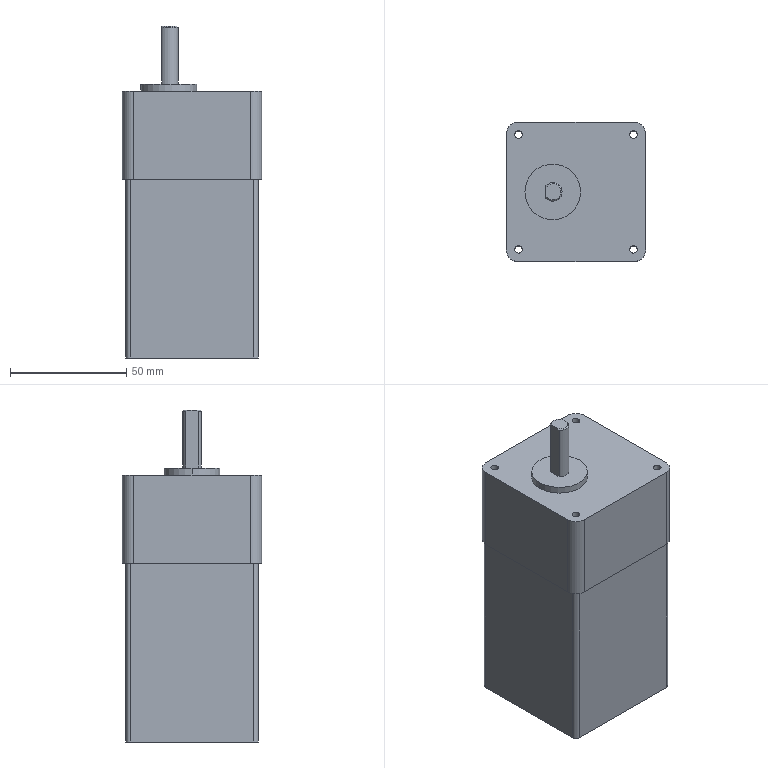Part | STEP file | 57BYG gear reduction stepper motor Mingren MR57BYG76-P10-1 | 1 solid | 34 faces | box 60 x 60 x 143 mm | volume 384480 mm3 | cylinder 19 | plane 14 | cone 1 | commonest cylinder face diameters 3.3 x8 4 x4 10 x4 24 x2 8 x1
STEP:
#1=CARTESIAN_POINT('',(-26.4,24.75,0.));
#2=VERTEX_POINT('',#1);
#3=CARTESIAN_POINT('',(-23.1,24.75,0.));
#4=VERTEX_POINT('',#3);
#5=CARTESIAN_POINT('',(-24.75,24.75,0.));
#6=DIRECTION('',(0.,0.,1.));
#7=DIRECTION('',(1.,0.,0.));
#8=AXIS2_PLACEMENT_3D('',#5,#6,#7);
#9=CIRCLE('',#8,1.65);
#10=EDGE_CURVE('',#2,#4,#9,.T.);
#11=ORIENTED_EDGE('',*,*,#10,.F.);
#12=CARTESIAN_POINT('',(-26.4,24.75,115.));
#13=VERTEX_POINT('',#12);
#14=CARTESIAN_POINT('',(-26.4,24.75,115.));
#15=DIRECTION('',(0.,0.,1.));
#16=VECTOR('',#15,1000.);
#17=LINE('',#14,#16);
#18=EDGE_CURVE('',#2,#13,#17,.T.);
#19=ORIENTED_EDGE('',*,*,#18,.T.);
#20=CARTESIAN_POINT('',(-23.1,24.75,115.));
#21=VERTEX_POINT('',#20);
#22=CARTESIAN_POINT('',(-24.75,24.75,115.));
#23=DIRECTION('',(0.,0.,1.));
#24=DIRECTION('',(1.,0.,0.));
#25=AXIS2_PLACEMENT_3D('',#22,#23,#24);
#26=CIRCLE('',#25,1.65);
#27=EDGE_CURVE('',#13,#21,#26,.T.);
#28=ORIENTED_EDGE('',*,*,#27,.T.);
#29=CARTESIAN_POINT('',(-23.1,24.75,115.));
#30=DIRECTION('',(0.,0.,1.));
#31=VECTOR('',#30,1000.);
#32=LINE('',#29,#31);
#33=EDGE_CURVE('',#4,#21,#32,.T.);
#34=ORIENTED_EDGE('',*,*,#33,.F.);
#35=EDGE_LOOP('',(#11,#19,#28,#34));
#36=FACE_OUTER_BOUND('',#35,.T.);
#37=CARTESIAN_POINT('',(-24.75,24.75,115.));
#38=DIRECTION('',(0.,0.,1.));
#39=DIRECTION('',(1.,0.,0.));
#40=AXIS2_PLACEMENT_3D('',#37,#38,#39);
#41=CYLINDRICAL_SURFACE('',#40,1.65);
#42=ADVANCED_FACE('',(#36),#41,.F.);
#43=CARTESIAN_POINT('',(23.1,24.75,0.));
#44=VERTEX_POINT('',#43);
#45=CARTESIAN_POINT('',(26.4,24.75,0.));
#46=VERTEX_POINT('',#45);
#47=CARTESIAN_POINT('',(24.75,24.75,0.));
#48=DIRECTION('',(0.,0.,1.));
#49=DIRECTION('',(1.,0.,0.));
#50=AXIS2_PLACEMENT_3D('',#47,#48,#49);
#51=CIRCLE('',#50,1.65);
#52=EDGE_CURVE('',#44,#46,#51,.T.);
#53=ORIENTED_EDGE('',*,*,#52,.F.);
#54=CARTESIAN_POINT('',(23.1,24.75,115.));
#55=VERTEX_POINT('',#54);
#56=CARTESIAN_POINT('',(23.1,24.75,115.));
#57=DIRECTION('',(0.,0.,1.));
#58=VECTOR('',#57,1000.);
#59=LINE('',#56,#58);
#60=EDGE_CURVE('',#44,#55,#59,.T.);
#61=ORIENTED_EDGE('',*,*,#60,.T.);
#62=CARTESIAN_POINT('',(26.4,24.75,115.));
#63=VERTEX_POINT('',#62);
#64=CARTESIAN_POINT('',(24.75,24.75,115.));
#65=DIRECTION('',(0.,0.,1.));
#66=DIRECTION('',(1.,0.,0.));
#67=AXIS2_PLACEMENT_3D('',#64,#65,#66);
#68=CIRCLE('',#67,1.65);
#69=EDGE_CURVE('',#55,#63,#68,.T.);
#70=ORIENTED_EDGE('',*,*,#69,.T.);
#71=CARTESIAN_POINT('',(26.4,24.75,115.));
#72=DIRECTION('',(0.,0.,1.));
#73=VECTOR('',#72,1000.);
#74=LINE('',#71,#73);
#75=EDGE_CURVE('',#46,#63,#74,.T.);
#76=ORIENTED_EDGE('',*,*,#75,.F.);
#77=EDGE_LOOP('',(#53,#61,#70,#76));
#78=FACE_OUTER_BOUND('',#77,.T.);
#79=CARTESIAN_POINT('',(24.75,24.75,115.));
#80=DIRECTION('',(0.,0.,1.));
#81=DIRECTION('',(1.,0.,0.));
#82=AXIS2_PLACEMENT_3D('',#79,#80,#81);
#83=CYLINDRICAL_SURFACE('',#82,1.65);
#84=ADVANCED_FACE('',(#78),#83,.F.);
#85=CARTESIAN_POINT('',(23.1,-24.75,0.));
#86=VERTEX_POINT('',#85);
#87=CARTESIAN_POINT('',(26.4,-24.75,0.));
#88=VERTEX_POINT('',#87);
#89=CARTESIAN_POINT('',(24.75,-24.75,0.));
#90=DIRECTION('',(0.,0.,1.));
#91=DIRECTION('',(1.,0.,0.));
#92=AXIS2_PLACEMENT_3D('',#89,#90,#91);
#93=CIRCLE('',#92,1.65);
#94=EDGE_CURVE('',#86,#88,#93,.T.);
#95=ORIENTED_EDGE('',*,*,#94,.F.);
#96=CARTESIAN_POINT('',(23.1,-24.75,115.));
#97=VERTEX_POINT('',#96);
#98=CARTESIAN_POINT('',(23.1,-24.75,115.));
#99=DIRECTION('',(0.,0.,1.));
#100=VECTOR('',#99,1000.);
#101=LINE('',#98,#100);
#102=EDGE_CURVE('',#86,#97,#101,.T.);
#103=ORIENTED_EDGE('',*,*,#102,.T.);
#104=CARTESIAN_POINT('',(26.4,-24.75,115.));
#105=VERTEX_POINT('',#104);
#106=CARTESIAN_POINT('',(24.75,-24.75,115.));
#107=DIRECTION('',(0.,0.,1.));
#108=DIRECTION('',(1.,0.,0.));
#109=AXIS2_PLACEMENT_3D('',#106,#107,#108);
#110=CIRCLE('',#109,1.65);
#111=EDGE_CURVE('',#97,#105,#110,.T.);
#112=ORIENTED_EDGE('',*,*,#111,.T.);
#113=CARTESIAN_POINT('',(26.4,-24.75,115.));
#114=DIRECTION('',(0.,0.,1.));
#115=VECTOR('',#114,1000.);
#116=LINE('',#113,#115);
#117=EDGE_CURVE('',#88,#105,#116,.T.);
#118=ORIENTED_EDGE('',*,*,#117,.F.);
#119=EDGE_LOOP('',(#95,#103,#112,#118));
#120=FACE_OUTER_BOUND('',#119,.T.);
#121=CARTESIAN_POINT('',(24.75,-24.75,115.));
#122=DIRECTION('',(0.,0.,1.));
#123=DIRECTION('',(1.,0.,0.));
#124=AXIS2_PLACEMENT_3D('',#121,#122,#123);
#125=CYLINDRICAL_SURFACE('',#124,1.65);
#126=ADVANCED_FACE('',(#120),#125,.F.);
#127=CARTESIAN_POINT('',(-26.4,-24.75,0.));
#128=VERTEX_POINT('',#127);
#129=CARTESIAN_POINT('',(-23.1,-24.75,0.));
#130=VERTEX_POINT('',#129);
#131=CARTESIAN_POINT('',(-24.75,-24.75,0.));
#132=DIRECTION('',(0.,0.,1.));
#133=DIRECTION('',(1.,0.,0.));
#134=AXIS2_PLACEMENT_3D('',#131,#132,#133);
#135=CIRCLE('',#134,1.65);
#136=EDGE_CURVE('',#128,#130,#135,.T.);
#137=ORIENTED_EDGE('',*,*,#136,.F.);
#138=CARTESIAN_POINT('',(-26.4,-24.75,115.));
#139=VERTEX_POINT('',#138);
#140=CARTESIAN_POINT('',(-26.4,-24.75,115.));
#141=DIRECTION('',(0.,0.,1.));
#142=VECTOR('',#141,1000.);
#143=LINE('',#140,#142);
#144=EDGE_CURVE('',#128,#139,#143,.T.);
#145=ORIENTED_EDGE('',*,*,#144,.T.);
#146=CARTESIAN_POINT('',(-23.1,-24.75,115.));
#147=VERTEX_POINT('',#146);
#148=CARTESIAN_POINT('',(-24.75,-24.75,115.));
#149=DIRECTION('',(0.,0.,1.));
#150=DIRECTION('',(1.,0.,0.));
#151=AXIS2_PLACEMENT_3D('',#148,#149,#150);
#152=CIRCLE('',#151,1.65);
#153=EDGE_CURVE('',#139,#147,#152,.T.);
#154=ORIENTED_EDGE('',*,*,#153,.T.);
#155=CARTESIAN_POINT('',(-23.1,-24.75,115.));
#156=DIRECTION('',(0.,0.,1.));
#157=VECTOR('',#156,1000.);
#158=LINE('',#155,#157);
#159=EDGE_CURVE('',#130,#147,#158,.T.);
#160=ORIENTED_EDGE('',*,*,#159,.F.);
#161=EDGE_LOOP('',(#137,#145,#154,#160));
#162=FACE_OUTER_BOUND('',#161,.T.);
#163=CARTESIAN_POINT('',(-24.75,-24.75,115.));
#164=DIRECTION('',(0.,0.,1.));
#165=DIRECTION('',(1.,0.,0.));
#166=AXIS2_PLACEMENT_3D('',#163,#164,#165);
#167=CYLINDRICAL_SURFACE('',#166,1.65);
#168=ADVANCED_FACE('',(#162),#167,.F.);
#169=CARTESIAN_POINT('',(2.,0.,118.));
#170=VERTEX_POINT('',#169);
#171=CARTESIAN_POINT('',(-22.,0.,118.));
#172=VERTEX_POINT('',#171);
#173=CARTESIAN_POINT('',(-10.,0.,118.));
#174=DIRECTION('',(0.,0.,1.));
#175=DIRECTION('',(1.,0.,0.));
#176=AXIS2_PLACEMENT_3D('',#173,#174,#175);
#177=CIRCLE('',#176,12.);
#178=EDGE_CURVE('',#170,#172,#177,.T.);
#179=ORIENTED_EDGE('',*,*,#178,.F.);
#180=CARTESIAN_POINT('',(2.,0.,115.));
#181=VERTEX_POINT('',#180);
#182=CARTESIAN_POINT('',(2.,0.,118.));
#183=DIRECTION('',(0.,0.,-1.));
#184=VECTOR('',#183,1000.);
#185=LINE('',#182,#184);
#186=EDGE_CURVE('',#170,#181,#185,.T.);
#187=ORIENTED_EDGE('',*,*,#186,.T.);
#188=CARTESIAN_POINT('',(-22.,0.,115.));
#189=VERTEX_POINT('',#188);
#190=CARTESIAN_POINT('',(-10.,0.,115.));
#191=DIRECTION('',(0.,0.,1.));
#192=DIRECTION('',(1.,0.,0.));
#193=AXIS2_PLACEMENT_3D('',#190,#191,#192);
#194=CIRCLE('',#193,12.);
#195=EDGE_CURVE('',#181,#189,#194,.T.);
#196=ORIENTED_EDGE('',*,*,#195,.T.);
#197=CARTESIAN_POINT('',(-22.,0.,118.));
#198=DIRECTION('',(0.,0.,-1.));
#199=VECTOR('',#198,1000.);
#200=LINE('',#197,#199);
#201=EDGE_CURVE('',#172,#189,#200,.T.);
#202=ORIENTED_EDGE('',*,*,#201,.F.);
#203=EDGE_LOOP('',(#179,#187,#196,#202));
#204=FACE_OUTER_BOUND('',#203,.T.);
#205=CARTESIAN_POINT('',(-10.,0.,118.));
#206=DIRECTION('',(0.,0.,-1.));
#207=DIRECTION('',(-1.,0.,0.));
#208=AXIS2_PLACEMENT_3D('',#205,#206,#207);
#209=CYLINDRICAL_SURFACE('',#208,12.);
#210=ADVANCED_FACE('',(#204),#209,.T.);
#211=CARTESIAN_POINT('',(-30.,-25.,77.));
#212=VERTEX_POINT('',#211);
#213=CARTESIAN_POINT('',(-30.,25.,77.));
#214=VERTEX_POINT('',#213);
#215=CARTESIAN_POINT('',(-30.,30.,77.));
#216=DIRECTION('',(0.,1.,0.));
#217=VECTOR('',#216,1000.);
#218=LINE('',#215,#217);
#219=EDGE_CURVE('',#212,#214,#218,.T.);
#220=ORIENTED_EDGE('',*,*,#219,.F.);
#221=CARTESIAN_POINT('',(-30.,-25.,115.));
#222=VERTEX_POINT('',#221);
#223=CARTESIAN_POINT('',(-30.,-25.,115.));
#224=DIRECTION('',(0.,0.,1.));
#225=VECTOR('',#224,1000.);
#226=LINE('',#223,#225);
#227=EDGE_CURVE('',#212,#222,#226,.T.);
#228=ORIENTED_EDGE('',*,*,#227,.T.);
#229=CARTESIAN_POINT('',(-30.,25.,115.));
#230=VERTEX_POINT('',#229);
#231=CARTESIAN_POINT('',(-30.,30.,115.));
#232=DIRECTION('',(0.,-1.,0.));
#233=VECTOR('',#232,1000.);
#234=LINE('',#231,#233);
#235=EDGE_CURVE('',#230,#222,#234,.T.);
#236=ORIENTED_EDGE('',*,*,#235,.F.);
#237=CARTESIAN_POINT('',(-30.,25.,115.));
#238=DIRECTION('',(0.,0.,-1.));
#239=VECTOR('',#238,1000.);
#240=LINE('',#237,#239);
#241=EDGE_CURVE('',#230,#214,#240,.T.);
#242=ORIENTED_EDGE('',*,*,#241,.T.);
#243=EDGE_LOOP('',(#220,#228,#236,#242));
#244=FACE_OUTER_BOUND('',#243,.T.);
#245=CARTESIAN_POINT('',(-30.,30.,115.));
#246=DIRECTION('',(1.,0.,0.));
#247=DIRECTION('',(0.,0.,-1.));
#248=AXIS2_PLACEMENT_3D('',#245,#246,#247);
#249=PLANE('',#248);
#250=ADVANCED_FACE('',(#244),#249,.F.);
#251=CARTESIAN_POINT('',(25.,-30.,77.));
#252=VERTEX_POINT('',#251);
#253=CARTESIAN_POINT('',(-25.,-30.,77.));
#254=VERTEX_POINT('',#253);
#255=CARTESIAN_POINT('',(-30.,-30.,77.));
#256=DIRECTION('',(-1.,0.,0.));
#257=VECTOR('',#256,1000.);
#258=LINE('',#255,#257);
#259=EDGE_CURVE('',#252,#254,#258,.T.);
#260=ORIENTED_EDGE('',*,*,#259,.F.);
#261=CARTESIAN_POINT('',(25.,-30.,115.));
#262=VERTEX_POINT('',#261);
#263=CARTESIAN_POINT('',(25.,-30.,115.));
#264=DIRECTION('',(0.,0.,1.));
#265=VECTOR('',#264,1000.);
#266=LINE('',#263,#265);
#267=EDGE_CURVE('',#252,#262,#266,.T.);
#268=ORIENTED_EDGE('',*,*,#267,.T.);
#269=CARTESIAN_POINT('',(-25.,-30.,115.));
#270=VERTEX_POINT('',#269);
#271=CARTESIAN_POINT('',(-30.,-30.,115.));
#272=DIRECTION('',(1.,0.,0.));
#273=VECTOR('',#272,1000.);
#274=LINE('',#271,#273);
#275=EDGE_CURVE('',#270,#262,#274,.T.);
#276=ORIENTED_EDGE('',*,*,#275,.F.);
#277=CARTESIAN_POINT('',(-25.,-30.,115.));
#278=DIRECTION('',(0.,0.,-1.));
#279=VECTOR('',#278,1000.);
#280=LINE('',#277,#279);
#281=EDGE_CURVE('',#270,#254,#280,.T.);
#282=ORIENTED_EDGE('',*,*,#281,.T.);
#283=EDGE_LOOP('',(#260,#268,#276,#282));
#284=FACE_OUTER_BOUND('',#283,.T.);
#285=CARTESIAN_POINT('',(-30.,-30.,115.));
#286=DIRECTION('',(0.,1.,0.));
#287=DIRECTION('',(0.,0.,1.));
#288=AXIS2_PLACEMENT_3D('',#285,#286,#287);
#289=PLANE('',#288);
#290=ADVANCED_FACE('',(#284),#289,.F.);
#291=CARTESIAN_POINT('',(30.,25.,77.));
#292=VERTEX_POINT('',#291);
#293=CARTESIAN_POINT('',(30.,-25.,77.));
#294=VERTEX_POINT('',#293);
#295=CARTESIAN_POINT('',(30.,30.,77.));
#296=DIRECTION('',(0.,-1.,0.));
#297=VECTOR('',#296,1000.);
#298=LINE('',#295,#297);
#299=EDGE_CURVE('',#292,#294,#298,.T.);
#300=ORIENTED_EDGE('',*,*,#299,.F.);
#301=CARTESIAN_POINT('',(30.,25.,115.));
#302=VERTEX_POINT('',#301);
#303=CARTESIAN_POINT('',(30.,25.,115.));
#304=DIRECTION('',(0.,0.,1.));
#305=VECTOR('',#304,1000.);
#306=LINE('',#303,#305);
#307=EDGE_CURVE('',#292,#302,#306,.T.);
#308=ORIENTED_EDGE('',*,*,#307,.T.);
#309=CARTESIAN_POINT('',(30.,-25.,115.));
#310=VERTEX_POINT('',#309);
#311=CARTESIAN_POINT('',(30.,30.,115.));
#312=DIRECTION('',(0.,1.,0.));
#313=VECTOR('',#312,1000.);
#314=LINE('',#311,#313);
#315=EDGE_CURVE('',#310,#302,#314,.T.);
#316=ORIENTED_EDGE('',*,*,#315,.F.);
#317=CARTESIAN_POINT('',(30.,-25.,115.));
#318=DIRECTION('',(0.,0.,-1.));
#319=VECTOR('',#318,1000.);
#320=LINE('',#317,#319);
#321=EDGE_CURVE('',#310,#294,#320,.T.);
#322=ORIENTED_EDGE('',*,*,#321,.T.);
#323=EDGE_LOOP('',(#300,#308,#316,#322));
#324=FACE_OUTER_BOUND('',#323,.T.);
#325=CARTESIAN_POINT('',(30.,30.,115.));
#326=DIRECTION('',(-1.,0.,0.));
#327=DIRECTION('',(0.,0.,1.));
#328=AXIS2_PLACEMENT_3D('',#325,#326,#327);
#329=PLANE('',#328);
#330=ADVANCED_FACE('',(#324),#329,.F.);
#331=CARTESIAN_POINT('',(-25.,30.,77.));
#332=VERTEX_POINT('',#331);
#333=CARTESIAN_POINT('',(25.,30.,77.));
#334=VERTEX_POINT('',#333);
#335=CARTESIAN_POINT('',(-30.,30.,77.));
#336=DIRECTION('',(1.,0.,0.));
#337=VECTOR('',#336,1000.);
#338=LINE('',#335,#337);
#339=EDGE_CURVE('',#332,#334,#338,.T.);
#340=ORIENTED_EDGE('',*,*,#339,.F.);
#341=CARTESIAN_POINT('',(-25.,30.,115.));
#342=VERTEX_POINT('',#341);
#343=CARTESIAN_POINT('',(-25.,30.,115.));
#344=DIRECTION('',(0.,0.,1.));
#345=VECTOR('',#344,1000.);
#346=LINE('',#343,#345);
#347=EDGE_CURVE('',#332,#342,#346,.T.);
#348=ORIENTED_EDGE('',*,*,#347,.T.);
#349=CARTESIAN_POINT('',(25.,30.,115.));
#350=VERTEX_POINT('',#349);
#351=CARTESIAN_POINT('',(-30.,30.,115.));
#352=DIRECTION('',(-1.,0.,0.));
#353=VECTOR('',#352,1000.);
#354=LINE('',#351,#353);
#355=EDGE_CURVE('',#350,#342,#354,.T.);
#356=ORIENTED_EDGE('',*,*,#355,.F.);
#357=CARTESIAN_POINT('',(25.,30.,115.));
#358=DIRECTION('',(0.,0.,-1.));
#359=VECTOR('',#358,1000.);
#360=LINE('',#357,#359);
#361=EDGE_CURVE('',#350,#334,#360,.T.);
#362=ORIENTED_EDGE('',*,*,#361,.T.);
#363=EDGE_LOOP('',(#340,#348,#356,#362));
#364=FACE_OUTER_BOUND('',#363,.T.);
#365=CARTESIAN_POINT('',(-30.,30.,115.));
#366=DIRECTION('',(0.,-1.,0.));
#367=DIRECTION('',(0.,0.,-1.));
#368=AXIS2_PLACEMENT_3D('',#365,#366,#367);
#369=PLANE('',#368);
#370=ADVANCED_FACE('',(#364),#369,.F.);
#371=ORIENTED_EDGE('',*,*,#227,.F.);
#372=CARTESIAN_POINT('',(-25.,-25.,77.));
#373=DIRECTION('',(0.,0.,1.));
#374=DIRECTION('',(-1.,0.,0.));
#375=AXIS2_PLACEMENT_3D('',#372,#373,#374);
#376=CIRCLE('',#375,5.);
#377=EDGE_CURVE('',#212,#254,#376,.T.);
#378=ORIENTED_EDGE('',*,*,#377,.T.);
#379=ORIENTED_EDGE('',*,*,#281,.F.);
#380=CARTESIAN_POINT('',(-25.,-25.,115.));
#381=DIRECTION('',(0.,0.,1.));
#382=DIRECTION('',(1.,0.,0.));
#383=AXIS2_PLACEMENT_3D('',#380,#381,#382);
#384=CIRCLE('',#383,5.);
#385=EDGE_CURVE('',#222,#270,#384,.T.);
#386=ORIENTED_EDGE('',*,*,#385,.F.);
#387=EDGE_LOOP('',(#371,#378,#379,#386));
#388=FACE_OUTER_BOUND('',#387,.T.);
#389=CARTESIAN_POINT('',(-25.,-25.,115.));
#390=DIRECTION('',(0.,0.,-1.));
#391=DIRECTION('',(-1.,0.,0.));
#392=AXIS2_PLACEMENT_3D('',#389,#390,#391);
#393=CYLINDRICAL_SURFACE('',#392,5.);
#394=ADVANCED_FACE('',(#388),#393,.T.);
#395=ORIENTED_EDGE('',*,*,#267,.F.);
#396=CARTESIAN_POINT('',(25.,-25.,77.));
#397=DIRECTION('',(0.,0.,1.));
#398=DIRECTION('',(-1.,0.,0.));
#399=AXIS2_PLACEMENT_3D('',#396,#397,#398);
#400=CIRCLE('',#399,5.);
#401=EDGE_CURVE('',#252,#294,#400,.T.);
#402=ORIENTED_EDGE('',*,*,#401,.T.);
#403=ORIENTED_EDGE('',*,*,#321,.F.);
#404=CARTESIAN_POINT('',(25.,-25.,115.));
#405=DIRECTION('',(0.,0.,1.));
#406=DIRECTION('',(1.,0.,0.));
#407=AXIS2_PLACEMENT_3D('',#404,#405,#406);
#408=CIRCLE('',#407,5.);
#409=EDGE_CURVE('',#262,#310,#408,.T.);
#410=ORIENTED_EDGE('',*,*,#409,.F.);
#411=EDGE_LOOP('',(#395,#402,#403,#410));
#412=FACE_OUTER_BOUND('',#411,.T.);
#413=CARTESIAN_POINT('',(25.,-25.,115.));
#414=DIRECTION('',(0.,0.,-1.));
#415=DIRECTION('',(-1.,0.,0.));
#416=AXIS2_PLACEMENT_3D('',#413,#414,#415);
#417=CYLINDRICAL_SURFACE('',#416,5.);
#418=ADVANCED_FACE('',(#412),#417,.T.);
#419=ORIENTED_EDGE('',*,*,#307,.F.);
#420=CARTESIAN_POINT('',(25.,25.,77.));
#421=DIRECTION('',(0.,0.,1.));
#422=DIRECTION('',(-1.,0.,0.));
#423=AXIS2_PLACEMENT_3D('',#420,#421,#422);
#424=CIRCLE('',#423,5.);
#425=EDGE_CURVE('',#292,#334,#424,.T.);
#426=ORIENTED_EDGE('',*,*,#425,.T.);
#427=ORIENTED_EDGE('',*,*,#361,.F.);
#428=CARTESIAN_POINT('',(25.,25.,115.));
#429=DIRECTION('',(0.,0.,1.));
#430=DIRECTION('',(1.,0.,0.));
#431=AXIS2_PLACEMENT_3D('',#428,#429,#430);
#432=CIRCLE('',#431,5.);
#433=EDGE_CURVE('',#302,#350,#432,.T.);
#434=ORIENTED_EDGE('',*,*,#433,.F.);
#435=EDGE_LOOP('',(#419,#426,#427,#434));
#436=FACE_OUTER_BOUND('',#435,.T.);
#437=CARTESIAN_POINT('',(25.,25.,115.));
#438=DIRECTION('',(0.,0.,-1.));
#439=DIRECTION('',(-1.,0.,0.));
#440=AXIS2_PLACEMENT_3D('',#437,#438,#439);
#441=CYLINDRICAL_SURFACE('',#440,5.);
#442=ADVANCED_FACE('',(#436),#441,.T.);
#443=ORIENTED_EDGE('',*,*,#347,.F.);
#444=CARTESIAN_POINT('',(-25.,25.,77.));
#445=DIRECTION('',(0.,0.,1.));
#446=DIRECTION('',(-1.,0.,0.));
#447=AXIS2_PLACEMENT_3D('',#444,#445,#446);
#448=CIRCLE('',#447,5.);
#449=EDGE_CURVE('',#332,#214,#448,.T.);
#450=ORIENTED_EDGE('',*,*,#449,.T.);
#451=ORIENTED_EDGE('',*,*,#241,.F.);
#452=CARTESIAN_POINT('',(-25.,25.,115.));
#453=DIRECTION('',(0.,0.,1.));
#454=DIRECTION('',(1.,0.,0.));
#455=AXIS2_PLACEMENT_3D('',#452,#453,#454);
#456=CIRCLE('',#455,5.);
#457=EDGE_CURVE('',#342,#230,#456,.T.);
#458=ORIENTED_EDGE('',*,*,#457,.F.);
#459=EDGE_LOOP('',(#443,#450,#451,#458));
#460=FACE_OUTER_BOUND('',#459,.T.);
#461=CARTESIAN_POINT('',(-25.,25.,115.));
#462=DIRECTION('',(0.,0.,-1.));
#463=DIRECTION('',(-1.,0.,0.));
#464=AXIS2_PLACEMENT_3D('',#461,#462,#463);
#465=CYLINDRICAL_SURFACE('',#464,5.);
#466=ADVANCED_FACE('',(#460),#465,.T.);
#467=CARTESIAN_POINT('',(-24.75,24.75,115.));
#468=DIRECTION('',(0.,0.,1.));
#469=DIRECTION('',(1.,0.,0.));
#470=AXIS2_PLACEMENT_3D('',#467,#468,#469);
#471=CIRCLE('',#470,1.65);
#472=EDGE_CURVE('',#21,#13,#471,.T.);
#473=ORIENTED_EDGE('',*,*,#472,.F.);
#474=ORIENTED_EDGE('',*,*,#27,.F.);
#475=EDGE_LOOP('',(#473,#474));
#476=FACE_BOUND('',#475,.T.);
#477=CARTESIAN_POINT('',(24.75,24.75,115.));
#478=DIRECTION('',(0.,0.,1.));
#479=DIRECTION('',(1.,0.,0.));
#480=AXIS2_PLACEMENT_3D('',#477,#478,#479);
#481=CIRCLE('',#480,1.65);
#482=EDGE_CURVE('',#63,#55,#481,.T.);
#483=ORIENTED_EDGE('',*,*,#482,.F.);
#484=ORIENTED_EDGE('',*,*,#69,.F.);
#485=EDGE_LOOP('',(#483,#484));
#486=FACE_BOUND('',#485,.T.);
#487=CARTESIAN_POINT('',(24.75,-24.75,115.));
#488=DIRECTION('',(0.,0.,1.));
#489=DIRECTION('',(1.,0.,0.));
#490=AXIS2_PLACEMENT_3D('',#487,#488,#489);
#491=CIRCLE('',#490,1.65);
#492=EDGE_CURVE('',#105,#97,#491,.T.);
#493=ORIENTED_EDGE('',*,*,#492,.F.);
#494=ORIENTED_EDGE('',*,*,#111,.F.);
#495=EDGE_LOOP('',(#493,#494));
#496=FACE_BOUND('',#495,.T.);
#497=CARTESIAN_POINT('',(-24.75,-24.75,115.));
#498=DIRECTION('',(0.,0.,1.));
#499=DIRECTION('',(1.,0.,0.));
#500=AXIS2_PLACEMENT_3D('',#497,#498,#499);
#501=CIRCLE('',#500,1.65);
#502=EDGE_CURVE('',#147,#139,#501,.T.);
#503=ORIENTED_EDGE('',*,*,#502,.F.);
#504=ORIENTED_EDGE('',*,*,#153,.F.);
#505=EDGE_LOOP('',(#503,#504));
#506=FACE_BOUND('',#505,.T.);
#507=ORIENTED_EDGE('',*,*,#235,.T.);
#508=ORIENTED_EDGE('',*,*,#385,.T.);
#509=ORIENTED_EDGE('',*,*,#275,.T.);
#510=ORIENTED_EDGE('',*,*,#409,.T.);
#511=ORIENTED_EDGE('',*,*,#315,.T.);
#512=ORIENTED_EDGE('',*,*,#433,.T.);
#513=ORIENTED_EDGE('',*,*,#355,.T.);
#514=ORIENTED_EDGE('',*,*,#457,.T.);
#515=EDGE_LOOP('',(#507,#508,#509,#510,#511,#512,#513,#514));
#516=FACE_OUTER_BOUND('',#515,.T.);
#517=CARTESIAN_POINT('',(-10.,0.,115.));
#518=DIRECTION('',(0.,0.,1.));
#519=DIRECTION('',(1.,0.,0.));
#520=AXIS2_PLACEMENT_3D('',#517,#518,#519);
#521=CIRCLE('',#520,12.);
#522=EDGE_CURVE('',#189,#181,#521,.T.);
#523=ORIENTED_EDGE('',*,*,#522,.F.);
#524=ORIENTED_EDGE('',*,*,#195,.F.);
#525=EDGE_LOOP('',(#523,#524));
#526=FACE_BOUND('',#525,.T.);
#527=CARTESIAN_POINT('',(-30.,-30.,115.));
#528=DIRECTION('',(0.,0.,1.));
#529=DIRECTION('',(1.,0.,0.));
#530=AXIS2_PLACEMENT_3D('',#527,#528,#529);
#531=PLANE('',#530);
#532=ADVANCED_FACE('',(#476,#486,#496,#506,#516,#526),#531,.T.);
#533=CARTESIAN_POINT('',(-13.,-2.646,118.));
#534=VERTEX_POINT('',#533);
#535=CARTESIAN_POINT('',(-13.,2.646,118.));
#536=VERTEX_POINT('',#535);
#537=CARTESIAN_POINT('',(-10.,0.,118.));
#538=DIRECTION('',(0.,0.,1.));
#539=DIRECTION('',(1.,0.,0.));
#540=AXIS2_PLACEMENT_3D('',#537,#538,#539);
#541=CIRCLE('',#540,4.);
#542=EDGE_CURVE('',#534,#536,#541,.T.);
#543=ORIENTED_EDGE('',*,*,#542,.F.);
#544=CARTESIAN_POINT('',(-13.,5.,118.));
#545=DIRECTION('',(0.,1.,0.));
#546=VECTOR('',#545,1000.);
#547=LINE('',#544,#546);
#548=EDGE_CURVE('',#534,#536,#547,.T.);
#549=ORIENTED_EDGE('',*,*,#548,.T.);
#550=EDGE_LOOP('',(#543,#549));
#551=FACE_BOUND('',#550,.T.);
#552=CARTESIAN_POINT('',(-10.,0.,118.));
#553=DIRECTION('',(0.,0.,1.));
#554=DIRECTION('',(1.,0.,0.));
#555=AXIS2_PLACEMENT_3D('',#552,#553,#554);
#556=CIRCLE('',#555,12.);
#557=EDGE_CURVE('',#172,#170,#556,.T.);
#558=ORIENTED_EDGE('',*,*,#557,.T.);
#559=ORIENTED_EDGE('',*,*,#178,.T.);
#560=EDGE_LOOP('',(#558,#559));
#561=FACE_OUTER_BOUND('',#560,.T.);
#562=CARTESIAN_POINT('',(-10.,0.,118.));
#563=DIRECTION('',(0.,0.,1.));
#564=DIRECTION('',(1.,0.,0.));
#565=AXIS2_PLACEMENT_3D('',#562,#563,#564);
#566=PLANE('',#565);
#567=ADVANCED_FACE('',(#551,#561),#566,.T.);
#568=ORIENTED_EDGE('',*,*,#186,.F.);
#569=ORIENTED_EDGE('',*,*,#557,.F.);
#570=ORIENTED_EDGE('',*,*,#201,.T.);
#571=ORIENTED_EDGE('',*,*,#522,.T.);
#572=EDGE_LOOP('',(#568,#569,#570,#571));
#573=FACE_OUTER_BOUND('',#572,.T.);
#574=CARTESIAN_POINT('',(-10.,0.,118.));
#575=DIRECTION('',(0.,0.,-1.));
#576=DIRECTION('',(-1.,0.,0.));
#577=AXIS2_PLACEMENT_3D('',#574,#575,#576);
#578=CYLINDRICAL_SURFACE('',#577,12.);
#579=ADVANCED_FACE('',(#573),#578,.T.);
#580=CARTESIAN_POINT('',(-13.,-1.803,143.));
#581=VERTEX_POINT('',#580);
#582=CARTESIAN_POINT('',(-13.,1.803,143.));
#583=VERTEX_POINT('',#582);
#584=CARTESIAN_POINT('',(-13.,5.,143.));
#585=DIRECTION('',(0.,1.,0.));
#586=VECTOR('',#585,1000.);
#587=LINE('',#584,#586);
#588=EDGE_CURVE('',#581,#583,#587,.T.);
#589=ORIENTED_EDGE('',*,*,#588,.F.);
#590=CARTESIAN_POINT('',(-10.,0.,143.));
#591=DIRECTION('',(0.,0.,1.));
#592=DIRECTION('',(1.,0.,0.));
#593=AXIS2_PLACEMENT_3D('',#590,#591,#592);
#594=CIRCLE('',#593,3.5);
#595=EDGE_CURVE('',#581,#583,#594,.T.);
#596=ORIENTED_EDGE('',*,*,#595,.T.);
#597=EDGE_LOOP('',(#589,#596));
#598=FACE_OUTER_BOUND('',#597,.T.);
#599=CARTESIAN_POINT('',(-10.,0.,143.));
#600=DIRECTION('',(0.,0.,1.));
#601=DIRECTION('',(1.,0.,0.));
#602=AXIS2_PLACEMENT_3D('',#599,#600,#601);
#603=PLANE('',#602);
#604=ADVANCED_FACE('',(#598),#603,.T.);
#605=CARTESIAN_POINT('',(-13.,2.646,142.5));
#606=VERTEX_POINT('',#605);
#607=CARTESIAN_POINT('',(-13.,-2.646,142.5));
#608=VERTEX_POINT('',#607);
#609=CARTESIAN_POINT('',(-10.,0.,142.5));
#610=DIRECTION('',(0.,0.,-1.));
#611=DIRECTION('',(1.,0.,0.));
#612=AXIS2_PLACEMENT_3D('',#609,#610,#611);
#613=CIRCLE('',#612,4.);
#614=EDGE_CURVE('',#606,#608,#613,.T.);
#615=ORIENTED_EDGE('',*,*,#614,.T.);
#616=CARTESIAN_POINT('',(-13.,-2.646,143.));
#617=DIRECTION('',(0.,0.,-1.));
#618=VECTOR('',#617,1000.);
#619=LINE('',#616,#618);
#620=EDGE_CURVE('',#608,#534,#619,.T.);
#621=ORIENTED_EDGE('',*,*,#620,.T.);
#622=ORIENTED_EDGE('',*,*,#542,.T.);
#623=CARTESIAN_POINT('',(-13.,2.646,143.));
#624=DIRECTION('',(0.,0.,1.));
#625=VECTOR('',#624,1000.);
#626=LINE('',#623,#625);
#627=EDGE_CURVE('',#536,#606,#626,.T.);
#628=ORIENTED_EDGE('',*,*,#627,.T.);
#629=EDGE_LOOP('',(#615,#621,#622,#628));
#630=FACE_OUTER_BOUND('',#629,.T.);
#631=CARTESIAN_POINT('',(-10.,0.,143.));
#632=DIRECTION('',(0.,0.,-1.));
#633=DIRECTION('',(-1.,0.,0.));
#634=AXIS2_PLACEMENT_3D('',#631,#632,#633);
#635=CYLINDRICAL_SURFACE('',#634,4.);
#636=ADVANCED_FACE('',(#630),#635,.T.);
#637=CARTESIAN_POINT('',(-13.,-2.646,142.5));
#638=CARTESIAN_POINT('',(-13.,-2.374,142.68));
#639=CARTESIAN_POINT('',(-13.,-2.095,142.849));
#640=CARTESIAN_POINT('',(-13.,-1.803,143.));
#641=B_SPLINE_CURVE_WITH_KNOTS('',3,(#637,#638,#639,#640),.UNSPECIFIED.,.F.,.F.,(4,4),(0.007424,0.008405),.UNSPECIFIED.);
#642=EDGE_CURVE('',#608,#581,#641,.T.);
#643=ORIENTED_EDGE('',*,*,#642,.F.);
#644=ORIENTED_EDGE('',*,*,#614,.F.);
#645=CARTESIAN_POINT('',(-13.,1.803,143.));
#646=CARTESIAN_POINT('',(-13.,2.092,142.851));
#647=CARTESIAN_POINT('',(-13.,2.373,142.68));
#648=CARTESIAN_POINT('',(-13.,2.646,142.5));
#649=B_SPLINE_CURVE_WITH_KNOTS('',3,(#645,#646,#647,#648),.UNSPECIFIED.,.F.,.F.,(4,4),(0.01215,0.01313),.UNSPECIFIED.);
#650=EDGE_CURVE('',#583,#606,#649,.T.);
#651=ORIENTED_EDGE('',*,*,#650,.F.);
#652=ORIENTED_EDGE('',*,*,#595,.F.);
#653=EDGE_LOOP('',(#643,#644,#651,#652));
#654=FACE_OUTER_BOUND('',#653,.T.);
#655=CARTESIAN_POINT('',(-10.,0.,143.));
#656=DIRECTION('',(0.,0.,-1.));
#657=DIRECTION('',(-1.,0.,0.));
#658=AXIS2_PLACEMENT_3D('',#655,#656,#657);
#659=CONICAL_SURFACE('',#658,3.5,0.7854);
#660=ADVANCED_FACE('',(#654),#659,.T.);
#661=ORIENTED_EDGE('',*,*,#642,.T.);
#662=ORIENTED_EDGE('',*,*,#588,.T.);
#663=ORIENTED_EDGE('',*,*,#650,.T.);
#664=ORIENTED_EDGE('',*,*,#627,.F.);
#665=ORIENTED_EDGE('',*,*,#548,.F.);
#666=ORIENTED_EDGE('',*,*,#620,.F.);
#667=EDGE_LOOP('',(#661,#662,#663,#664,#665,#666));
#668=FACE_OUTER_BOUND('',#667,.T.);
#669=CARTESIAN_POINT('',(-13.,5.,118.));
#670=DIRECTION('',(1.,0.,0.));
#671=DIRECTION('',(0.,0.,-1.));
#672=AXIS2_PLACEMENT_3D('',#669,#670,#671);
#673=PLANE('',#672);
#674=ADVANCED_FACE('',(#668),#673,.F.);
#675=ORIENTED_EDGE('',*,*,#259,.T.);
#676=ORIENTED_EDGE('',*,*,#377,.F.);
#677=ORIENTED_EDGE('',*,*,#219,.T.);
#678=ORIENTED_EDGE('',*,*,#449,.F.);
#679=ORIENTED_EDGE('',*,*,#339,.T.);
#680=ORIENTED_EDGE('',*,*,#425,.F.);
#681=ORIENTED_EDGE('',*,*,#299,.T.);
#682=ORIENTED_EDGE('',*,*,#401,.F.);
#683=EDGE_LOOP('',(#675,#676,#677,#678,#679,#680,#681,#682));
#684=FACE_OUTER_BOUND('',#683,.T.);
#685=CARTESIAN_POINT('',(26.5,-28.5,77.));
#686=VERTEX_POINT('',#685);
#687=CARTESIAN_POINT('',(-26.5,-28.5,77.));
#688=VERTEX_POINT('',#687);
#689=CARTESIAN_POINT('',(28.5,-28.5,77.));
#690=DIRECTION('',(-1.,0.,0.));
#691=VECTOR('',#690,1000.);
#692=LINE('',#689,#691);
#693=EDGE_CURVE('',#686,#688,#692,.T.);
#694=ORIENTED_EDGE('',*,*,#693,.F.);
#695=CARTESIAN_POINT('',(28.5,-26.5,77.));
#696=VERTEX_POINT('',#695);
#697=CARTESIAN_POINT('',(26.5,-26.5,77.));
#698=DIRECTION('',(0.,0.,1.));
#699=DIRECTION('',(-1.,0.,0.));
#700=AXIS2_PLACEMENT_3D('',#697,#698,#699);
#701=CIRCLE('',#700,2.);
#702=EDGE_CURVE('',#686,#696,#701,.T.);
#703=ORIENTED_EDGE('',*,*,#702,.T.);
#704=CARTESIAN_POINT('',(28.5,26.5,77.));
#705=VERTEX_POINT('',#704);
#706=CARTESIAN_POINT('',(28.5,28.5,77.));
#707=DIRECTION('',(0.,-1.,0.));
#708=VECTOR('',#707,1000.);
#709=LINE('',#706,#708);
#710=EDGE_CURVE('',#705,#696,#709,.T.);
#711=ORIENTED_EDGE('',*,*,#710,.F.);
#712=CARTESIAN_POINT('',(26.5,28.5,77.));
#713=VERTEX_POINT('',#712);
#714=CARTESIAN_POINT('',(26.5,26.5,77.));
#715=DIRECTION('',(0.,0.,1.));
#716=DIRECTION('',(-1.,0.,0.));
#717=AXIS2_PLACEMENT_3D('',#714,#715,#716);
#718=CIRCLE('',#717,2.);
#719=EDGE_CURVE('',#705,#713,#718,.T.);
#720=ORIENTED_EDGE('',*,*,#719,.T.);
#721=CARTESIAN_POINT('',(-26.5,28.5,77.));
#722=VERTEX_POINT('',#721);
#723=CARTESIAN_POINT('',(28.5,28.5,77.));
#724=DIRECTION('',(1.,0.,0.));
#725=VECTOR('',#724,1000.);
#726=LINE('',#723,#725);
#727=EDGE_CURVE('',#722,#713,#726,.T.);
#728=ORIENTED_EDGE('',*,*,#727,.F.);
#729=CARTESIAN_POINT('',(-28.5,26.5,77.));
#730=VERTEX_POINT('',#729);
#731=CARTESIAN_POINT('',(-26.5,26.5,77.));
#732=DIRECTION('',(0.,0.,1.));
#733=DIRECTION('',(-1.,0.,0.));
#734=AXIS2_PLACEMENT_3D('',#731,#732,#733);
#735=CIRCLE('',#734,2.);
#736=EDGE_CURVE('',#722,#730,#735,.T.);
#737=ORIENTED_EDGE('',*,*,#736,.T.);
#738=CARTESIAN_POINT('',(-28.5,-26.5,77.));
#739=VERTEX_POINT('',#738);
#740=CARTESIAN_POINT('',(-28.5,28.5,77.));
#741=DIRECTION('',(0.,1.,0.));
#742=VECTOR('',#741,1000.);
#743=LINE('',#740,#742);
#744=EDGE_CURVE('',#739,#730,#743,.T.);
#745=ORIENTED_EDGE('',*,*,#744,.F.);
#746=CARTESIAN_POINT('',(-26.5,-26.5,77.));
#747=DIRECTION('',(0.,0.,1.));
#748=DIRECTION('',(-1.,0.,0.));
#749=AXIS2_PLACEMENT_3D('',#746,#747,#748);
#750=CIRCLE('',#749,2.);
#751=EDGE_CURVE('',#739,#688,#750,.T.);
#752=ORIENTED_EDGE('',*,*,#751,.T.);
#753=EDGE_LOOP('',(#694,#703,#711,#720,#728,#737,#745,#752));
#754=FACE_BOUND('',#753,.T.);
#755=CARTESIAN_POINT('',(0.,0.,77.));
#756=DIRECTION('',(0.,0.,-1.));
#757=DIRECTION('',(-1.,0.,0.));
#758=AXIS2_PLACEMENT_3D('',#755,#756,#757);
#759=PLANE('',#758);
#760=ADVANCED_FACE('',(#684,#754),#759,.T.);
#761=CARTESIAN_POINT('',(-28.5,-26.5,0.));
#762=VERTEX_POINT('',#761);
#763=CARTESIAN_POINT('',(-28.5,26.5,0.));
#764=VERTEX_POINT('',#763);
#765=CARTESIAN_POINT('',(-28.5,28.5,0.));
#766=DIRECTION('',(0.,1.,0.));
#767=VECTOR('',#766,1000.);
#768=LINE('',#765,#767);
#769=EDGE_CURVE('',#762,#764,#768,.T.);
#770=ORIENTED_EDGE('',*,*,#769,.F.);
#771=CARTESIAN_POINT('',(-28.5,-26.5,77.));
#772=DIRECTION('',(0.,0.,1.));
#773=VECTOR('',#772,1000.);
#774=LINE('',#771,#773);
#775=EDGE_CURVE('',#762,#739,#774,.T.);
#776=ORIENTED_EDGE('',*,*,#775,.T.);
#777=ORIENTED_EDGE('',*,*,#744,.T.);
#778=CARTESIAN_POINT('',(-28.5,26.5,77.));
#779=DIRECTION('',(0.,0.,-1.));
#780=VECTOR('',#779,1000.);
#781=LINE('',#778,#780);
#782=EDGE_CURVE('',#730,#764,#781,.T.);
#783=ORIENTED_EDGE('',*,*,#782,.T.);
#784=EDGE_LOOP('',(#770,#776,#777,#783));
#785=FACE_OUTER_BOUND('',#784,.T.);
#786=CARTESIAN_POINT('',(-28.5,28.5,77.));
#787=DIRECTION('',(-1.,0.,0.));
#788=DIRECTION('',(0.,-1.,0.));
#789=AXIS2_PLACEMENT_3D('',#786,#787,#788);
#790=PLANE('',#789);
#791=ADVANCED_FACE('',(#785),#790,.T.);
#792=ORIENTED_EDGE('',*,*,#693,.T.);
#793=CARTESIAN_POINT('',(-26.5,-28.5,0.));
#794=VERTEX_POINT('',#793);
#795=CARTESIAN_POINT('',(-26.5,-28.5,77.));
#796=DIRECTION('',(0.,0.,-1.));
#797=VECTOR('',#796,1000.);
#798=LINE('',#795,#797);
#799=EDGE_CURVE('',#688,#794,#798,.T.);
#800=ORIENTED_EDGE('',*,*,#799,.T.);
#801=CARTESIAN_POINT('',(26.5,-28.5,0.));
#802=VERTEX_POINT('',#801);
#803=CARTESIAN_POINT('',(28.5,-28.5,0.));
#804=DIRECTION('',(-1.,0.,0.));
#805=VECTOR('',#804,1000.);
#806=LINE('',#803,#805);
#807=EDGE_CURVE('',#802,#794,#806,.T.);
#808=ORIENTED_EDGE('',*,*,#807,.F.);
#809=CARTESIAN_POINT('',(26.5,-28.5,77.));
#810=DIRECTION('',(0.,0.,1.));
#811=VECTOR('',#810,1000.);
#812=LINE('',#809,#811);
#813=EDGE_CURVE('',#802,#686,#812,.T.);
#814=ORIENTED_EDGE('',*,*,#813,.T.);
#815=EDGE_LOOP('',(#792,#800,#808,#814));
#816=FACE_OUTER_BOUND('',#815,.T.);
#817=CARTESIAN_POINT('',(28.5,-28.5,77.));
#818=DIRECTION('',(0.,-1.,0.));
#819=DIRECTION('',(0.,0.,-1.));
#820=AXIS2_PLACEMENT_3D('',#817,#818,#819);
#821=PLANE('',#820);
#822=ADVANCED_FACE('',(#816),#821,.T.);
#823=ORIENTED_EDGE('',*,*,#710,.T.);
#824=CARTESIAN_POINT('',(28.5,-26.5,0.));
#825=VERTEX_POINT('',#824);
#826=CARTESIAN_POINT('',(28.5,-26.5,77.));
#827=DIRECTION('',(0.,0.,-1.));
#828=VECTOR('',#827,1000.);
#829=LINE('',#826,#828);
#830=EDGE_CURVE('',#696,#825,#829,.T.);
#831=ORIENTED_EDGE('',*,*,#830,.T.);
#832=CARTESIAN_POINT('',(28.5,26.5,0.));
#833=VERTEX_POINT('',#832);
#834=CARTESIAN_POINT('',(28.5,28.5,0.));
#835=DIRECTION('',(0.,-1.,0.));
#836=VECTOR('',#835,1000.);
#837=LINE('',#834,#836);
#838=EDGE_CURVE('',#833,#825,#837,.T.);
#839=ORIENTED_EDGE('',*,*,#838,.F.);
#840=CARTESIAN_POINT('',(28.5,26.5,77.));
#841=DIRECTION('',(0.,0.,1.));
#842=VECTOR('',#841,1000.);
#843=LINE('',#840,#842);
#844=EDGE_CURVE('',#833,#705,#843,.T.);
#845=ORIENTED_EDGE('',*,*,#844,.T.);
#846=EDGE_LOOP('',(#823,#831,#839,#845));
#847=FACE_OUTER_BOUND('',#846,.T.);
#848=CARTESIAN_POINT('',(28.5,28.5,77.));
#849=DIRECTION('',(1.,0.,0.));
#850=DIRECTION('',(0.,1.,0.));
#851=AXIS2_PLACEMENT_3D('',#848,#849,#850);
#852=PLANE('',#851);
#853=ADVANCED_FACE('',(#847),#852,.T.);
#854=ORIENTED_EDGE('',*,*,#727,.T.);
#855=CARTESIAN_POINT('',(26.5,28.5,0.));
#856=VERTEX_POINT('',#855);
#857=CARTESIAN_POINT('',(26.5,28.5,77.));
#858=DIRECTION('',(0.,0.,-1.));
#859=VECTOR('',#858,1000.);
#860=LINE('',#857,#859);
#861=EDGE_CURVE('',#713,#856,#860,.T.);
#862=ORIENTED_EDGE('',*,*,#861,.T.);
#863=CARTESIAN_POINT('',(-26.5,28.5,0.));
#864=VERTEX_POINT('',#863);
#865=CARTESIAN_POINT('',(28.5,28.5,0.));
#866=DIRECTION('',(1.,0.,0.));
#867=VECTOR('',#866,1000.);
#868=LINE('',#865,#867);
#869=EDGE_CURVE('',#864,#856,#868,.T.);
#870=ORIENTED_EDGE('',*,*,#869,.F.);
#871=CARTESIAN_POINT('',(-26.5,28.5,77.));
#872=DIRECTION('',(0.,0.,1.));
#873=VECTOR('',#872,1000.);
#874=LINE('',#871,#873);
#875=EDGE_CURVE('',#864,#722,#874,.T.);
#876=ORIENTED_EDGE('',*,*,#875,.T.);
#877=EDGE_LOOP('',(#854,#862,#870,#876));
#878=FACE_OUTER_BOUND('',#877,.T.);
#879=CARTESIAN_POINT('',(28.5,28.5,77.));
#880=DIRECTION('',(0.,1.,0.));
#881=DIRECTION('',(0.,0.,1.));
#882=AXIS2_PLACEMENT_3D('',#879,#880,#881);
#883=PLANE('',#882);
#884=ADVANCED_FACE('',(#878),#883,.T.);
#885=CARTESIAN_POINT('',(-24.75,24.75,0.));
#886=DIRECTION('',(0.,0.,1.));
#887=DIRECTION('',(1.,0.,0.));
#888=AXIS2_PLACEMENT_3D('',#885,#886,#887);
#889=CIRCLE('',#888,1.65);
#890=EDGE_CURVE('',#4,#2,#889,.T.);
#891=ORIENTED_EDGE('',*,*,#890,.T.);
#892=ORIENTED_EDGE('',*,*,#10,.T.);
#893=EDGE_LOOP('',(#891,#892));
#894=FACE_BOUND('',#893,.T.);
#895=CARTESIAN_POINT('',(24.75,24.75,0.));
#896=DIRECTION('',(0.,0.,1.));
#897=DIRECTION('',(1.,0.,0.));
#898=AXIS2_PLACEMENT_3D('',#895,#896,#897);
#899=CIRCLE('',#898,1.65);
#900=EDGE_CURVE('',#46,#44,#899,.T.);
#901=ORIENTED_EDGE('',*,*,#900,.T.);
#902=ORIENTED_EDGE('',*,*,#52,.T.);
#903=EDGE_LOOP('',(#901,#902));
#904=FACE_BOUND('',#903,.T.);
#905=CARTESIAN_POINT('',(24.75,-24.75,0.));
#906=DIRECTION('',(0.,0.,1.));
#907=DIRECTION('',(1.,0.,0.));
#908=AXIS2_PLACEMENT_3D('',#905,#906,#907);
#909=CIRCLE('',#908,1.65);
#910=EDGE_CURVE('',#88,#86,#909,.T.);
#911=ORIENTED_EDGE('',*,*,#910,.T.);
#912=ORIENTED_EDGE('',*,*,#94,.T.);
#913=EDGE_LOOP('',(#911,#912));
#914=FACE_BOUND('',#913,.T.);
#915=CARTESIAN_POINT('',(-24.75,-24.75,0.));
#916=DIRECTION('',(0.,0.,1.));
#917=DIRECTION('',(1.,0.,0.));
#918=AXIS2_PLACEMENT_3D('',#915,#916,#917);
#919=CIRCLE('',#918,1.65);
#920=EDGE_CURVE('',#130,#128,#919,.T.);
#921=ORIENTED_EDGE('',*,*,#920,.T.);
#922=ORIENTED_EDGE('',*,*,#136,.T.);
#923=EDGE_LOOP('',(#921,#922));
#924=FACE_BOUND('',#923,.T.);
#925=ORIENTED_EDGE('',*,*,#807,.T.);
#926=CARTESIAN_POINT('',(-26.5,-26.5,0.));
#927=DIRECTION('',(0.,0.,-1.));
#928=DIRECTION('',(1.,0.,0.));
#929=AXIS2_PLACEMENT_3D('',#926,#927,#928);
#930=CIRCLE('',#929,2.);
#931=EDGE_CURVE('',#794,#762,#930,.T.);
#932=ORIENTED_EDGE('',*,*,#931,.T.);
#933=ORIENTED_EDGE('',*,*,#769,.T.);
#934=CARTESIAN_POINT('',(-26.5,26.5,0.));
#935=DIRECTION('',(0.,0.,-1.));
#936=DIRECTION('',(1.,0.,0.));
#937=AXIS2_PLACEMENT_3D('',#934,#935,#936);
#938=CIRCLE('',#937,2.);
#939=EDGE_CURVE('',#764,#864,#938,.T.);
#940=ORIENTED_EDGE('',*,*,#939,.T.);
#941=ORIENTED_EDGE('',*,*,#869,.T.);
#942=CARTESIAN_POINT('',(26.5,26.5,0.));
#943=DIRECTION('',(0.,0.,-1.));
#944=DIRECTION('',(1.,0.,0.));
#945=AXIS2_PLACEMENT_3D('',#942,#943,#944);
#946=CIRCLE('',#945,2.);
#947=EDGE_CURVE('',#856,#833,#946,.T.);
#948=ORIENTED_EDGE('',*,*,#947,.T.);
#949=ORIENTED_EDGE('',*,*,#838,.T.);
#950=CARTESIAN_POINT('',(26.5,-26.5,0.));
#951=DIRECTION('',(0.,0.,-1.));
#952=DIRECTION('',(1.,0.,0.));
#953=AXIS2_PLACEMENT_3D('',#950,#951,#952);
#954=CIRCLE('',#953,2.);
#955=EDGE_CURVE('',#825,#802,#954,.T.);
#956=ORIENTED_EDGE('',*,*,#955,.T.);
#957=EDGE_LOOP('',(#925,#932,#933,#940,#941,#948,#949,#956));
#958=FACE_OUTER_BOUND('',#957,.T.);
#959=CARTESIAN_POINT('',(-30.,-30.,0.));
#960=DIRECTION('',(0.,0.,1.));
#961=DIRECTION('',(1.,0.,0.));
#962=AXIS2_PLACEMENT_3D('',#959,#960,#961);
#963=PLANE('',#962);
#964=ADVANCED_FACE('',(#894,#904,#914,#924,#958),#963,.F.);
#965=ORIENTED_EDGE('',*,*,#144,.F.);
#966=ORIENTED_EDGE('',*,*,#920,.F.);
#967=ORIENTED_EDGE('',*,*,#159,.T.);
#968=ORIENTED_EDGE('',*,*,#502,.T.);
#969=EDGE_LOOP('',(#965,#966,#967,#968));
#970=FACE_OUTER_BOUND('',#969,.T.);
#971=CARTESIAN_POINT('',(-24.75,-24.75,115.));
#972=DIRECTION('',(0.,0.,1.));
#973=DIRECTION('',(1.,0.,0.));
#974=AXIS2_PLACEMENT_3D('',#971,#972,#973);
#975=CYLINDRICAL_SURFACE('',#974,1.65);
#976=ADVANCED_FACE('',(#970),#975,.F.);
#977=ORIENTED_EDGE('',*,*,#102,.F.);
#978=ORIENTED_EDGE('',*,*,#910,.F.);
#979=ORIENTED_EDGE('',*,*,#117,.T.);
#980=ORIENTED_EDGE('',*,*,#492,.T.);
#981=EDGE_LOOP('',(#977,#978,#979,#980));
#982=FACE_OUTER_BOUND('',#981,.T.);
#983=CARTESIAN_POINT('',(24.75,-24.75,115.));
#984=DIRECTION('',(0.,0.,1.));
#985=DIRECTION('',(1.,0.,0.));
#986=AXIS2_PLACEMENT_3D('',#983,#984,#985);
#987=CYLINDRICAL_SURFACE('',#986,1.65);
#988=ADVANCED_FACE('',(#982),#987,.F.);
#989=ORIENTED_EDGE('',*,*,#60,.F.);
#990=ORIENTED_EDGE('',*,*,#900,.F.);
#991=ORIENTED_EDGE('',*,*,#75,.T.);
#992=ORIENTED_EDGE('',*,*,#482,.T.);
#993=EDGE_LOOP('',(#989,#990,#991,#992));
#994=FACE_OUTER_BOUND('',#993,.T.);
#995=CARTESIAN_POINT('',(24.75,24.75,115.));
#996=DIRECTION('',(0.,0.,1.));
#997=DIRECTION('',(1.,0.,0.));
#998=AXIS2_PLACEMENT_3D('',#995,#996,#997);
#999=CYLINDRICAL_SURFACE('',#998,1.65);
#1000=ADVANCED_FACE('',(#994),#999,.F.);
#1001=ORIENTED_EDGE('',*,*,#18,.F.);
#1002=ORIENTED_EDGE('',*,*,#890,.F.);
#1003=ORIENTED_EDGE('',*,*,#33,.T.);
#1004=ORIENTED_EDGE('',*,*,#472,.T.);
#1005=EDGE_LOOP('',(#1001,#1002,#1003,#1004));
#1006=FACE_OUTER_BOUND('',#1005,.T.);
#1007=CARTESIAN_POINT('',(-24.75,24.75,115.));
#1008=DIRECTION('',(0.,0.,1.));
#1009=DIRECTION('',(1.,0.,0.));
#1010=AXIS2_PLACEMENT_3D('',#1007,#1008,#1009);
#1011=CYLINDRICAL_SURFACE('',#1010,1.65);
#1012=ADVANCED_FACE('',(#1006),#1011,.F.);
#1013=ORIENTED_EDGE('',*,*,#751,.F.);
#1014=ORIENTED_EDGE('',*,*,#775,.F.);
#1015=ORIENTED_EDGE('',*,*,#931,.F.);
#1016=ORIENTED_EDGE('',*,*,#799,.F.);
#1017=EDGE_LOOP('',(#1013,#1014,#1015,#1016));
#1018=FACE_OUTER_BOUND('',#1017,.T.);
#1019=CARTESIAN_POINT('',(-26.5,-26.5,77.));
#1020=DIRECTION('',(0.,0.,-1.));
#1021=DIRECTION('',(-1.,0.,0.));
#1022=AXIS2_PLACEMENT_3D('',#1019,#1020,#1021);
#1023=CYLINDRICAL_SURFACE('',#1022,2.);
#1024=ADVANCED_FACE('',(#1018),#1023,.T.);
#1025=ORIENTED_EDGE('',*,*,#702,.F.);
#1026=ORIENTED_EDGE('',*,*,#813,.F.);
#1027=ORIENTED_EDGE('',*,*,#955,.F.);
#1028=ORIENTED_EDGE('',*,*,#830,.F.);
#1029=EDGE_LOOP('',(#1025,#1026,#1027,#1028));
#1030=FACE_OUTER_BOUND('',#1029,.T.);
#1031=CARTESIAN_POINT('',(26.5,-26.5,77.));
#1032=DIRECTION('',(0.,0.,-1.));
#1033=DIRECTION('',(-1.,0.,0.));
#1034=AXIS2_PLACEMENT_3D('',#1031,#1032,#1033);
#1035=CYLINDRICAL_SURFACE('',#1034,2.);
#1036=ADVANCED_FACE('',(#1030),#1035,.T.);
#1037=ORIENTED_EDGE('',*,*,#719,.F.);
#1038=ORIENTED_EDGE('',*,*,#844,.F.);
#1039=ORIENTED_EDGE('',*,*,#947,.F.);
#1040=ORIENTED_EDGE('',*,*,#861,.F.);
#1041=EDGE_LOOP('',(#1037,#1038,#1039,#1040));
#1042=FACE_OUTER_BOUND('',#1041,.T.);
#1043=CARTESIAN_POINT('',(26.5,26.5,77.));
#1044=DIRECTION('',(0.,0.,-1.));
#1045=DIRECTION('',(-1.,0.,0.));
#1046=AXIS2_PLACEMENT_3D('',#1043,#1044,#1045);
#1047=CYLINDRICAL_SURFACE('',#1046,2.);
#1048=ADVANCED_FACE('',(#1042),#1047,.T.);
#1049=ORIENTED_EDGE('',*,*,#736,.F.);
#1050=ORIENTED_EDGE('',*,*,#875,.F.);
#1051=ORIENTED_EDGE('',*,*,#939,.F.);
#1052=ORIENTED_EDGE('',*,*,#782,.F.);
#1053=EDGE_LOOP('',(#1049,#1050,#1051,#1052));
#1054=FACE_OUTER_BOUND('',#1053,.T.);
#1055=CARTESIAN_POINT('',(-26.5,26.5,77.));
#1056=DIRECTION('',(0.,0.,-1.));
#1057=DIRECTION('',(-1.,0.,0.));
#1058=AXIS2_PLACEMENT_3D('',#1055,#1056,#1057);
#1059=CYLINDRICAL_SURFACE('',#1058,2.);
#1060=ADVANCED_FACE('',(#1054),#1059,.T.);
#1061=CLOSED_SHELL('',(#42,#84,#126,#168,#210,#250,#290,#330,#370,#394,#418,#442,#466,#532,#567,#579,#604,#636,#660,#674,#760,#791,#822,#853,#884,#964,#976,#988,#1000,#1012,#1024,#1036,#1048,#1060));
#1062=MANIFOLD_SOLID_BREP('',#1061);
#1063=CARTESIAN_POINT('',(0.,0.,0.));
#1064=DIRECTION('',(0.,0.,1.));
#1065=DIRECTION('',(1.,0.,0.));
#1066=AXIS2_PLACEMENT_3D('',#1063,#1064,#1065);
#1067=(LENGTH_UNIT()NAMED_UNIT(*)SI_UNIT(.MILLI.,.METRE.));
#1068=UNCERTAINTY_MEASURE_WITH_UNIT(LENGTH_MEASURE(0.00001),#1067,'','');
#1069=(NAMED_UNIT(*)PLANE_ANGLE_UNIT()SI_UNIT($,.RADIAN.));
#1070=(NAMED_UNIT(*)SI_UNIT($,.STERADIAN.)SOLID_ANGLE_UNIT());
#1071=(GEOMETRIC_REPRESENTATION_CONTEXT(3)GLOBAL_UNCERTAINTY_ASSIGNED_CONTEXT((#1068))GLOBAL_UNIT_ASSIGNED_CONTEXT((#1067,#1069,#1070))REPRESENTATION_CONTEXT('',''));
#1072=ADVANCED_BREP_SHAPE_REPRESENTATION('',(#1062,#1066),#1071);